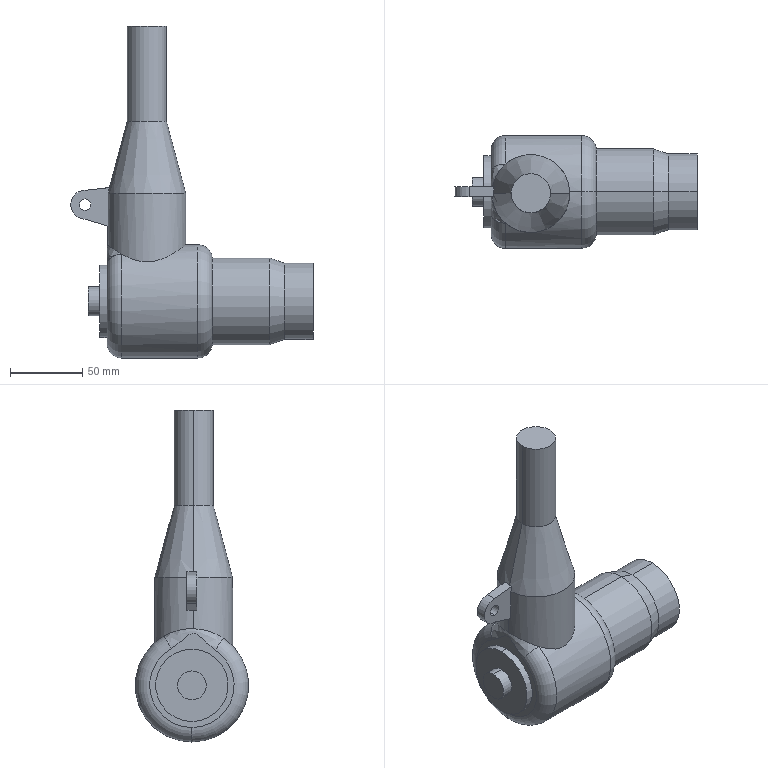Part | SolidWorks | features ICE 6, Fillet 2, Revolution 1 | 1 solid | 43 faces | box 168.244 x 78.608 x 230.304 mm | volume 658696 mm3 | cylinder 19 | plane 13 | cone 6 | torus 4 | spline 1 | commonest cylinder face diameters 20 x5 8 x2 27.205 x2 50.22 x2 53 x2 54 x2